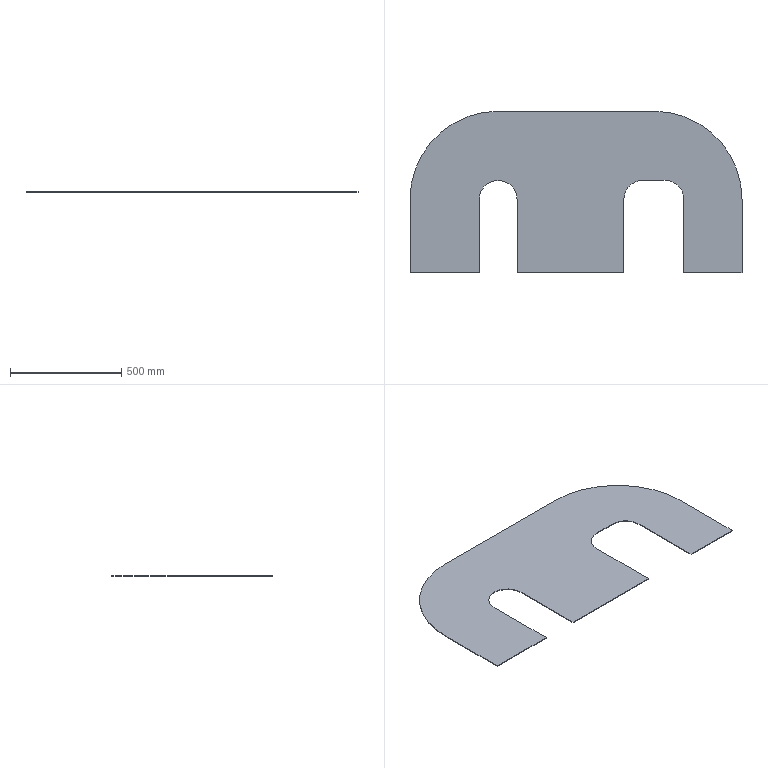Part | NX | features BREP 1 | 1 solid | 18 faces | box 1492 x 726 x 3 mm | volume 2518464 mm3 | plane 13 | cylinder 5 | commonest cylinder face diameters 170 x3 792 x2
STEP:
#1=CARTESIAN_POINT('',(-350.,396.,-1.5));
#2=VERTEX_POINT('',#1);
#3=CARTESIAN_POINT('',(-746.,0.,-1.5));
#4=VERTEX_POINT('',#3);
#5=CARTESIAN_POINT('',(-350.,0.,-1.5));
#6=DIRECTION('',(0.,0.,1.));
#7=DIRECTION('',(1.,0.,0.));
#8=AXIS2_PLACEMENT_3D('',#5,#6,#7);
#9=CIRCLE('',#8,396.);
#10=EDGE_CURVE('',#2,#4,#9,.T.);
#11=ORIENTED_EDGE('',*,*,#10,.T.);
#12=CARTESIAN_POINT('',(-746.,0.,1.5));
#13=VERTEX_POINT('',#12);
#14=CARTESIAN_POINT('',(-746.,0.,1.5));
#15=DIRECTION('',(0.,0.,-1.));
#16=VECTOR('',#15,1000.);
#17=LINE('',#14,#16);
#18=EDGE_CURVE('',#13,#4,#17,.T.);
#19=ORIENTED_EDGE('',*,*,#18,.F.);
#20=CARTESIAN_POINT('',(-350.,396.,1.5));
#21=VERTEX_POINT('',#20);
#22=CARTESIAN_POINT('',(-350.,0.,1.5));
#23=DIRECTION('',(0.,0.,1.));
#24=DIRECTION('',(1.,0.,0.));
#25=AXIS2_PLACEMENT_3D('',#22,#23,#24);
#26=CIRCLE('',#25,396.);
#27=EDGE_CURVE('',#21,#13,#26,.T.);
#28=ORIENTED_EDGE('',*,*,#27,.F.);
#29=CARTESIAN_POINT('',(-350.,396.,1.5));
#30=DIRECTION('',(0.,0.,-1.));
#31=VECTOR('',#30,1000.);
#32=LINE('',#29,#31);
#33=EDGE_CURVE('',#21,#2,#32,.T.);
#34=ORIENTED_EDGE('',*,*,#33,.T.);
#35=EDGE_LOOP('',(#11,#19,#28,#34));
#36=FACE_BOUND('',#35,.T.);
#37=CARTESIAN_POINT('',(-350.,0.,1.5));
#38=DIRECTION('',(0.,0.,-1.));
#39=DIRECTION('',(1.,0.,0.));
#40=AXIS2_PLACEMENT_3D('',#37,#38,#39);
#41=CYLINDRICAL_SURFACE('',#40,396.);
#42=ADVANCED_FACE('',(#36),#41,.T.);
#43=CARTESIAN_POINT('',(-746.,-330.,-1.5));
#44=VERTEX_POINT('',#43);
#45=CARTESIAN_POINT('',(-746.,0.,-1.5));
#46=DIRECTION('',(0.,-1.,0.));
#47=VECTOR('',#46,1000.);
#48=LINE('',#45,#47);
#49=EDGE_CURVE('',#4,#44,#48,.T.);
#50=ORIENTED_EDGE('',*,*,#49,.T.);
#51=CARTESIAN_POINT('',(-746.,-330.,1.5));
#52=VERTEX_POINT('',#51);
#53=CARTESIAN_POINT('',(-746.,-330.,1.5));
#54=DIRECTION('',(0.,0.,-1.));
#55=VECTOR('',#54,1000.);
#56=LINE('',#53,#55);
#57=EDGE_CURVE('',#52,#44,#56,.T.);
#58=ORIENTED_EDGE('',*,*,#57,.F.);
#59=CARTESIAN_POINT('',(-746.,0.,1.5));
#60=DIRECTION('',(0.,-1.,0.));
#61=VECTOR('',#60,1000.);
#62=LINE('',#59,#61);
#63=EDGE_CURVE('',#13,#52,#62,.T.);
#64=ORIENTED_EDGE('',*,*,#63,.F.);
#65=ORIENTED_EDGE('',*,*,#18,.T.);
#66=EDGE_LOOP('',(#50,#58,#64,#65));
#67=FACE_BOUND('',#66,.T.);
#68=CARTESIAN_POINT('',(-746.,0.,1.5));
#69=DIRECTION('',(1.,0.,0.));
#70=DIRECTION('',(0.,0.,1.));
#71=AXIS2_PLACEMENT_3D('',#68,#69,#70);
#72=PLANE('',#71);
#73=ADVANCED_FACE('',(#67),#72,.F.);
#74=CARTESIAN_POINT('',(-435.,-330.,-1.5));
#75=VERTEX_POINT('',#74);
#76=CARTESIAN_POINT('',(-746.,-330.,-1.5));
#77=DIRECTION('',(1.,0.,0.));
#78=VECTOR('',#77,1000.);
#79=LINE('',#76,#78);
#80=EDGE_CURVE('',#44,#75,#79,.T.);
#81=ORIENTED_EDGE('',*,*,#80,.T.);
#82=CARTESIAN_POINT('',(-435.,-330.,1.5));
#83=VERTEX_POINT('',#82);
#84=CARTESIAN_POINT('',(-435.,-330.,1.5));
#85=DIRECTION('',(0.,0.,-1.));
#86=VECTOR('',#85,1000.);
#87=LINE('',#84,#86);
#88=EDGE_CURVE('',#83,#75,#87,.T.);
#89=ORIENTED_EDGE('',*,*,#88,.F.);
#90=CARTESIAN_POINT('',(-746.,-330.,1.5));
#91=DIRECTION('',(1.,0.,0.));
#92=VECTOR('',#91,1000.);
#93=LINE('',#90,#92);
#94=EDGE_CURVE('',#52,#83,#93,.T.);
#95=ORIENTED_EDGE('',*,*,#94,.F.);
#96=ORIENTED_EDGE('',*,*,#57,.T.);
#97=EDGE_LOOP('',(#81,#89,#95,#96));
#98=FACE_BOUND('',#97,.T.);
#99=CARTESIAN_POINT('',(-746.,-330.,1.5));
#100=DIRECTION('',(0.,1.,0.));
#101=DIRECTION('',(1.,0.,0.));
#102=AXIS2_PLACEMENT_3D('',#99,#100,#101);
#103=PLANE('',#102);
#104=ADVANCED_FACE('',(#98),#103,.F.);
#105=CARTESIAN_POINT('',(-435.,0.,-1.5));
#106=VERTEX_POINT('',#105);
#107=CARTESIAN_POINT('',(-435.,0.,-1.5));
#108=DIRECTION('',(0.,1.,0.));
#109=VECTOR('',#108,1000.);
#110=LINE('',#107,#109);
#111=EDGE_CURVE('',#75,#106,#110,.T.);
#112=ORIENTED_EDGE('',*,*,#111,.T.);
#113=CARTESIAN_POINT('',(-435.,0.,1.5));
#114=VERTEX_POINT('',#113);
#115=CARTESIAN_POINT('',(-435.,0.,1.5));
#116=DIRECTION('',(0.,0.,-1.));
#117=VECTOR('',#116,1000.);
#118=LINE('',#115,#117);
#119=EDGE_CURVE('',#114,#106,#118,.T.);
#120=ORIENTED_EDGE('',*,*,#119,.F.);
#121=CARTESIAN_POINT('',(-435.,0.,1.5));
#122=DIRECTION('',(0.,1.,0.));
#123=VECTOR('',#122,1000.);
#124=LINE('',#121,#123);
#125=EDGE_CURVE('',#83,#114,#124,.T.);
#126=ORIENTED_EDGE('',*,*,#125,.F.);
#127=ORIENTED_EDGE('',*,*,#88,.T.);
#128=EDGE_LOOP('',(#112,#120,#126,#127));
#129=FACE_BOUND('',#128,.T.);
#130=CARTESIAN_POINT('',(-435.,0.,1.5));
#131=DIRECTION('',(-1.,0.,0.));
#132=DIRECTION('',(0.,1.,0.));
#133=AXIS2_PLACEMENT_3D('',#130,#131,#132);
#134=PLANE('',#133);
#135=ADVANCED_FACE('',(#129),#134,.F.);
#136=CARTESIAN_POINT('',(-265.,0.,-1.5));
#137=VERTEX_POINT('',#136);
#138=CARTESIAN_POINT('',(-350.,0.,-1.5));
#139=DIRECTION('',(0.,0.,-1.));
#140=DIRECTION('',(1.,0.,0.));
#141=AXIS2_PLACEMENT_3D('',#138,#139,#140);
#142=CIRCLE('',#141,85.);
#143=EDGE_CURVE('',#106,#137,#142,.T.);
#144=ORIENTED_EDGE('',*,*,#143,.T.);
#145=CARTESIAN_POINT('',(-265.,0.,1.5));
#146=VERTEX_POINT('',#145);
#147=CARTESIAN_POINT('',(-265.,0.,1.5));
#148=DIRECTION('',(0.,0.,-1.));
#149=VECTOR('',#148,1000.);
#150=LINE('',#147,#149);
#151=EDGE_CURVE('',#146,#137,#150,.T.);
#152=ORIENTED_EDGE('',*,*,#151,.F.);
#153=CARTESIAN_POINT('',(-350.,0.,1.5));
#154=DIRECTION('',(0.,0.,-1.));
#155=DIRECTION('',(1.,0.,0.));
#156=AXIS2_PLACEMENT_3D('',#153,#154,#155);
#157=CIRCLE('',#156,85.);
#158=EDGE_CURVE('',#114,#146,#157,.T.);
#159=ORIENTED_EDGE('',*,*,#158,.F.);
#160=ORIENTED_EDGE('',*,*,#119,.T.);
#161=EDGE_LOOP('',(#144,#152,#159,#160));
#162=FACE_BOUND('',#161,.T.);
#163=CARTESIAN_POINT('',(-350.,0.,1.5));
#164=DIRECTION('',(0.,0.,-1.));
#165=DIRECTION('',(1.,0.,0.));
#166=AXIS2_PLACEMENT_3D('',#163,#164,#165);
#167=CYLINDRICAL_SURFACE('',#166,85.);
#168=ADVANCED_FACE('',(#162),#167,.F.);
#169=CARTESIAN_POINT('',(-265.,-330.,-1.5));
#170=VERTEX_POINT('',#169);
#171=CARTESIAN_POINT('',(-265.,0.,-1.5));
#172=DIRECTION('',(0.,-1.,0.));
#173=VECTOR('',#172,1000.);
#174=LINE('',#171,#173);
#175=EDGE_CURVE('',#137,#170,#174,.T.);
#176=ORIENTED_EDGE('',*,*,#175,.T.);
#177=CARTESIAN_POINT('',(-265.,-330.,1.5));
#178=VERTEX_POINT('',#177);
#179=CARTESIAN_POINT('',(-265.,-330.,1.5));
#180=DIRECTION('',(0.,0.,-1.));
#181=VECTOR('',#180,1000.);
#182=LINE('',#179,#181);
#183=EDGE_CURVE('',#178,#170,#182,.T.);
#184=ORIENTED_EDGE('',*,*,#183,.F.);
#185=CARTESIAN_POINT('',(-265.,0.,1.5));
#186=DIRECTION('',(0.,-1.,0.));
#187=VECTOR('',#186,1000.);
#188=LINE('',#185,#187);
#189=EDGE_CURVE('',#146,#178,#188,.T.);
#190=ORIENTED_EDGE('',*,*,#189,.F.);
#191=ORIENTED_EDGE('',*,*,#151,.T.);
#192=EDGE_LOOP('',(#176,#184,#190,#191));
#193=FACE_BOUND('',#192,.T.);
#194=CARTESIAN_POINT('',(-265.,0.,1.5));
#195=DIRECTION('',(1.,0.,0.));
#196=DIRECTION('',(0.,-1.,0.));
#197=AXIS2_PLACEMENT_3D('',#194,#195,#196);
#198=PLANE('',#197);
#199=ADVANCED_FACE('',(#193),#198,.F.);
#200=CARTESIAN_POINT('',(215.,-330.,-1.5));
#201=VERTEX_POINT('',#200);
#202=CARTESIAN_POINT('',(-265.,-330.,-1.5));
#203=DIRECTION('',(1.,0.,0.));
#204=VECTOR('',#203,1000.);
#205=LINE('',#202,#204);
#206=EDGE_CURVE('',#170,#201,#205,.T.);
#207=ORIENTED_EDGE('',*,*,#206,.T.);
#208=CARTESIAN_POINT('',(215.,-330.,1.5));
#209=VERTEX_POINT('',#208);
#210=CARTESIAN_POINT('',(215.,-330.,1.5));
#211=DIRECTION('',(0.,0.,-1.));
#212=VECTOR('',#211,1000.);
#213=LINE('',#210,#212);
#214=EDGE_CURVE('',#209,#201,#213,.T.);
#215=ORIENTED_EDGE('',*,*,#214,.F.);
#216=CARTESIAN_POINT('',(-265.,-330.,1.5));
#217=DIRECTION('',(1.,0.,0.));
#218=VECTOR('',#217,1000.);
#219=LINE('',#216,#218);
#220=EDGE_CURVE('',#178,#209,#219,.T.);
#221=ORIENTED_EDGE('',*,*,#220,.F.);
#222=ORIENTED_EDGE('',*,*,#183,.T.);
#223=EDGE_LOOP('',(#207,#215,#221,#222));
#224=FACE_BOUND('',#223,.T.);
#225=CARTESIAN_POINT('',(-265.,-330.,1.5));
#226=DIRECTION('',(0.,1.,0.));
#227=DIRECTION('',(0.,0.,-1.));
#228=AXIS2_PLACEMENT_3D('',#225,#226,#227);
#229=PLANE('',#228);
#230=ADVANCED_FACE('',(#224),#229,.F.);
#231=CARTESIAN_POINT('',(215.,0.,-1.5));
#232=VERTEX_POINT('',#231);
#233=CARTESIAN_POINT('',(215.,0.,-1.5));
#234=DIRECTION('',(0.,1.,0.));
#235=VECTOR('',#234,1000.);
#236=LINE('',#233,#235);
#237=EDGE_CURVE('',#201,#232,#236,.T.);
#238=ORIENTED_EDGE('',*,*,#237,.T.);
#239=CARTESIAN_POINT('',(215.,0.,1.5));
#240=VERTEX_POINT('',#239);
#241=CARTESIAN_POINT('',(215.,0.,1.5));
#242=DIRECTION('',(0.,0.,-1.));
#243=VECTOR('',#242,1000.);
#244=LINE('',#241,#243);
#245=EDGE_CURVE('',#240,#232,#244,.T.);
#246=ORIENTED_EDGE('',*,*,#245,.F.);
#247=CARTESIAN_POINT('',(215.,0.,1.5));
#248=DIRECTION('',(0.,1.,0.));
#249=VECTOR('',#248,1000.);
#250=LINE('',#247,#249);
#251=EDGE_CURVE('',#209,#240,#250,.T.);
#252=ORIENTED_EDGE('',*,*,#251,.F.);
#253=ORIENTED_EDGE('',*,*,#214,.T.);
#254=EDGE_LOOP('',(#238,#246,#252,#253));
#255=FACE_BOUND('',#254,.T.);
#256=CARTESIAN_POINT('',(215.,0.,1.5));
#257=DIRECTION('',(-1.,0.,0.));
#258=DIRECTION('',(0.,1.,0.));
#259=AXIS2_PLACEMENT_3D('',#256,#257,#258);
#260=PLANE('',#259);
#261=ADVANCED_FACE('',(#255),#260,.F.);
#262=CARTESIAN_POINT('',(300.,85.,-1.5));
#263=VERTEX_POINT('',#262);
#264=CARTESIAN_POINT('',(300.,0.,-1.5));
#265=DIRECTION('',(0.,0.,-1.));
#266=DIRECTION('',(1.,0.,0.));
#267=AXIS2_PLACEMENT_3D('',#264,#265,#266);
#268=CIRCLE('',#267,85.);
#269=EDGE_CURVE('',#232,#263,#268,.T.);
#270=ORIENTED_EDGE('',*,*,#269,.T.);
#271=CARTESIAN_POINT('',(300.,85.,1.5));
#272=VERTEX_POINT('',#271);
#273=CARTESIAN_POINT('',(300.,85.,1.5));
#274=DIRECTION('',(0.,0.,-1.));
#275=VECTOR('',#274,1000.);
#276=LINE('',#273,#275);
#277=EDGE_CURVE('',#272,#263,#276,.T.);
#278=ORIENTED_EDGE('',*,*,#277,.F.);
#279=CARTESIAN_POINT('',(300.,0.,1.5));
#280=DIRECTION('',(0.,0.,-1.));
#281=DIRECTION('',(1.,0.,0.));
#282=AXIS2_PLACEMENT_3D('',#279,#280,#281);
#283=CIRCLE('',#282,85.);
#284=EDGE_CURVE('',#240,#272,#283,.T.);
#285=ORIENTED_EDGE('',*,*,#284,.F.);
#286=ORIENTED_EDGE('',*,*,#245,.T.);
#287=EDGE_LOOP('',(#270,#278,#285,#286));
#288=FACE_BOUND('',#287,.T.);
#289=CARTESIAN_POINT('',(300.,0.,1.5));
#290=DIRECTION('',(0.,0.,-1.));
#291=DIRECTION('',(1.,0.,0.));
#292=AXIS2_PLACEMENT_3D('',#289,#290,#291);
#293=CYLINDRICAL_SURFACE('',#292,85.);
#294=ADVANCED_FACE('',(#288),#293,.F.);
#295=CARTESIAN_POINT('',(400.,85.,-1.5));
#296=VERTEX_POINT('',#295);
#297=CARTESIAN_POINT('',(300.,85.,-1.5));
#298=DIRECTION('',(1.,0.,0.));
#299=VECTOR('',#298,1000.);
#300=LINE('',#297,#299);
#301=EDGE_CURVE('',#263,#296,#300,.T.);
#302=ORIENTED_EDGE('',*,*,#301,.T.);
#303=CARTESIAN_POINT('',(400.,85.,1.5));
#304=VERTEX_POINT('',#303);
#305=CARTESIAN_POINT('',(400.,85.,1.5));
#306=DIRECTION('',(0.,0.,-1.));
#307=VECTOR('',#306,1000.);
#308=LINE('',#305,#307);
#309=EDGE_CURVE('',#304,#296,#308,.T.);
#310=ORIENTED_EDGE('',*,*,#309,.F.);
#311=CARTESIAN_POINT('',(300.,85.,1.5));
#312=DIRECTION('',(1.,0.,0.));
#313=VECTOR('',#312,1000.);
#314=LINE('',#311,#313);
#315=EDGE_CURVE('',#272,#304,#314,.T.);
#316=ORIENTED_EDGE('',*,*,#315,.F.);
#317=ORIENTED_EDGE('',*,*,#277,.T.);
#318=EDGE_LOOP('',(#302,#310,#316,#317));
#319=FACE_BOUND('',#318,.T.);
#320=CARTESIAN_POINT('',(300.,85.,1.5));
#321=DIRECTION('',(0.,1.,0.));
#322=DIRECTION('',(0.,0.,-1.));
#323=AXIS2_PLACEMENT_3D('',#320,#321,#322);
#324=PLANE('',#323);
#325=ADVANCED_FACE('',(#319),#324,.F.);
#326=CARTESIAN_POINT('',(485.,0.,-1.5));
#327=VERTEX_POINT('',#326);
#328=CARTESIAN_POINT('',(400.,0.,-1.5));
#329=DIRECTION('',(0.,0.,-1.));
#330=DIRECTION('',(-1.,0.,0.));
#331=AXIS2_PLACEMENT_3D('',#328,#329,#330);
#332=CIRCLE('',#331,85.);
#333=EDGE_CURVE('',#296,#327,#332,.T.);
#334=ORIENTED_EDGE('',*,*,#333,.T.);
#335=CARTESIAN_POINT('',(485.,0.,1.5));
#336=VERTEX_POINT('',#335);
#337=CARTESIAN_POINT('',(485.,0.,1.5));
#338=DIRECTION('',(0.,0.,-1.));
#339=VECTOR('',#338,1000.);
#340=LINE('',#337,#339);
#341=EDGE_CURVE('',#336,#327,#340,.T.);
#342=ORIENTED_EDGE('',*,*,#341,.F.);
#343=CARTESIAN_POINT('',(400.,0.,1.5));
#344=DIRECTION('',(0.,0.,-1.));
#345=DIRECTION('',(-1.,0.,0.));
#346=AXIS2_PLACEMENT_3D('',#343,#344,#345);
#347=CIRCLE('',#346,85.);
#348=EDGE_CURVE('',#304,#336,#347,.T.);
#349=ORIENTED_EDGE('',*,*,#348,.F.);
#350=ORIENTED_EDGE('',*,*,#309,.T.);
#351=EDGE_LOOP('',(#334,#342,#349,#350));
#352=FACE_BOUND('',#351,.T.);
#353=CARTESIAN_POINT('',(400.,0.,1.5));
#354=DIRECTION('',(0.,0.,-1.));
#355=DIRECTION('',(1.,0.,0.));
#356=AXIS2_PLACEMENT_3D('',#353,#354,#355);
#357=CYLINDRICAL_SURFACE('',#356,85.);
#358=ADVANCED_FACE('',(#352),#357,.F.);
#359=CARTESIAN_POINT('',(485.,-330.,-1.5));
#360=VERTEX_POINT('',#359);
#361=CARTESIAN_POINT('',(485.,0.,-1.5));
#362=DIRECTION('',(0.,-1.,0.));
#363=VECTOR('',#362,1000.);
#364=LINE('',#361,#363);
#365=EDGE_CURVE('',#327,#360,#364,.T.);
#366=ORIENTED_EDGE('',*,*,#365,.T.);
#367=CARTESIAN_POINT('',(485.,-330.,1.5));
#368=VERTEX_POINT('',#367);
#369=CARTESIAN_POINT('',(485.,-330.,1.5));
#370=DIRECTION('',(0.,0.,-1.));
#371=VECTOR('',#370,1000.);
#372=LINE('',#369,#371);
#373=EDGE_CURVE('',#368,#360,#372,.T.);
#374=ORIENTED_EDGE('',*,*,#373,.F.);
#375=CARTESIAN_POINT('',(485.,0.,1.5));
#376=DIRECTION('',(0.,-1.,0.));
#377=VECTOR('',#376,1000.);
#378=LINE('',#375,#377);
#379=EDGE_CURVE('',#336,#368,#378,.T.);
#380=ORIENTED_EDGE('',*,*,#379,.F.);
#381=ORIENTED_EDGE('',*,*,#341,.T.);
#382=EDGE_LOOP('',(#366,#374,#380,#381));
#383=FACE_BOUND('',#382,.T.);
#384=CARTESIAN_POINT('',(485.,0.,1.5));
#385=DIRECTION('',(1.,0.,0.));
#386=DIRECTION('',(0.,0.,1.));
#387=AXIS2_PLACEMENT_3D('',#384,#385,#386);
#388=PLANE('',#387);
#389=ADVANCED_FACE('',(#383),#388,.F.);
#390=CARTESIAN_POINT('',(746.,-330.,-1.5));
#391=VERTEX_POINT('',#390);
#392=CARTESIAN_POINT('',(485.,-330.,-1.5));
#393=DIRECTION('',(1.,0.,0.));
#394=VECTOR('',#393,1000.);
#395=LINE('',#392,#394);
#396=EDGE_CURVE('',#360,#391,#395,.T.);
#397=ORIENTED_EDGE('',*,*,#396,.T.);
#398=CARTESIAN_POINT('',(746.,-330.,1.5));
#399=VERTEX_POINT('',#398);
#400=CARTESIAN_POINT('',(746.,-330.,1.5));
#401=DIRECTION('',(0.,0.,-1.));
#402=VECTOR('',#401,1000.);
#403=LINE('',#400,#402);
#404=EDGE_CURVE('',#399,#391,#403,.T.);
#405=ORIENTED_EDGE('',*,*,#404,.F.);
#406=CARTESIAN_POINT('',(485.,-330.,1.5));
#407=DIRECTION('',(1.,0.,0.));
#408=VECTOR('',#407,1000.);
#409=LINE('',#406,#408);
#410=EDGE_CURVE('',#368,#399,#409,.T.);
#411=ORIENTED_EDGE('',*,*,#410,.F.);
#412=ORIENTED_EDGE('',*,*,#373,.T.);
#413=EDGE_LOOP('',(#397,#405,#411,#412));
#414=FACE_BOUND('',#413,.T.);
#415=CARTESIAN_POINT('',(485.,-330.,1.5));
#416=DIRECTION('',(0.,1.,0.));
#417=DIRECTION('',(0.,0.,-1.));
#418=AXIS2_PLACEMENT_3D('',#415,#416,#417);
#419=PLANE('',#418);
#420=ADVANCED_FACE('',(#414),#419,.F.);
#421=CARTESIAN_POINT('',(746.,0.,-1.5));
#422=VERTEX_POINT('',#421);
#423=CARTESIAN_POINT('',(746.,0.,-1.5));
#424=DIRECTION('',(0.,1.,0.));
#425=VECTOR('',#424,1000.);
#426=LINE('',#423,#425);
#427=EDGE_CURVE('',#391,#422,#426,.T.);
#428=ORIENTED_EDGE('',*,*,#427,.T.);
#429=CARTESIAN_POINT('',(746.,0.,1.5));
#430=VERTEX_POINT('',#429);
#431=CARTESIAN_POINT('',(746.,0.,1.5));
#432=DIRECTION('',(0.,0.,-1.));
#433=VECTOR('',#432,1000.);
#434=LINE('',#431,#433);
#435=EDGE_CURVE('',#430,#422,#434,.T.);
#436=ORIENTED_EDGE('',*,*,#435,.F.);
#437=CARTESIAN_POINT('',(746.,0.,1.5));
#438=DIRECTION('',(0.,1.,0.));
#439=VECTOR('',#438,1000.);
#440=LINE('',#437,#439);
#441=EDGE_CURVE('',#399,#430,#440,.T.);
#442=ORIENTED_EDGE('',*,*,#441,.F.);
#443=ORIENTED_EDGE('',*,*,#404,.T.);
#444=EDGE_LOOP('',(#428,#436,#442,#443));
#445=FACE_BOUND('',#444,.T.);
#446=CARTESIAN_POINT('',(746.,0.,1.5));
#447=DIRECTION('',(-1.,0.,0.));
#448=DIRECTION('',(0.,0.,-1.));
#449=AXIS2_PLACEMENT_3D('',#446,#447,#448);
#450=PLANE('',#449);
#451=ADVANCED_FACE('',(#445),#450,.F.);
#452=CARTESIAN_POINT('',(350.,396.,-1.5));
#453=VERTEX_POINT('',#452);
#454=CARTESIAN_POINT('',(350.,0.,-1.5));
#455=DIRECTION('',(0.,0.,1.));
#456=DIRECTION('',(-1.,0.,0.));
#457=AXIS2_PLACEMENT_3D('',#454,#455,#456);
#458=CIRCLE('',#457,396.);
#459=EDGE_CURVE('',#422,#453,#458,.T.);
#460=ORIENTED_EDGE('',*,*,#459,.T.);
#461=CARTESIAN_POINT('',(350.,396.,1.5));
#462=VERTEX_POINT('',#461);
#463=CARTESIAN_POINT('',(350.,396.,1.5));
#464=DIRECTION('',(0.,0.,-1.));
#465=VECTOR('',#464,1000.);
#466=LINE('',#463,#465);
#467=EDGE_CURVE('',#462,#453,#466,.T.);
#468=ORIENTED_EDGE('',*,*,#467,.F.);
#469=CARTESIAN_POINT('',(350.,0.,1.5));
#470=DIRECTION('',(0.,0.,1.));
#471=DIRECTION('',(-1.,0.,0.));
#472=AXIS2_PLACEMENT_3D('',#469,#470,#471);
#473=CIRCLE('',#472,396.);
#474=EDGE_CURVE('',#430,#462,#473,.T.);
#475=ORIENTED_EDGE('',*,*,#474,.F.);
#476=ORIENTED_EDGE('',*,*,#435,.T.);
#477=EDGE_LOOP('',(#460,#468,#475,#476));
#478=FACE_BOUND('',#477,.T.);
#479=CARTESIAN_POINT('',(350.,0.,1.5));
#480=DIRECTION('',(0.,0.,-1.));
#481=DIRECTION('',(1.,0.,0.));
#482=AXIS2_PLACEMENT_3D('',#479,#480,#481);
#483=CYLINDRICAL_SURFACE('',#482,396.);
#484=ADVANCED_FACE('',(#478),#483,.T.);
#485=CARTESIAN_POINT('',(-350.,396.,-1.5));
#486=DIRECTION('',(-1.,0.,0.));
#487=VECTOR('',#486,1000.);
#488=LINE('',#485,#487);
#489=EDGE_CURVE('',#453,#2,#488,.T.);
#490=ORIENTED_EDGE('',*,*,#489,.T.);
#491=ORIENTED_EDGE('',*,*,#33,.F.);
#492=CARTESIAN_POINT('',(-350.,396.,1.5));
#493=DIRECTION('',(-1.,0.,0.));
#494=VECTOR('',#493,1000.);
#495=LINE('',#492,#494);
#496=EDGE_CURVE('',#462,#21,#495,.T.);
#497=ORIENTED_EDGE('',*,*,#496,.F.);
#498=ORIENTED_EDGE('',*,*,#467,.T.);
#499=EDGE_LOOP('',(#490,#491,#497,#498));
#500=FACE_BOUND('',#499,.T.);
#501=CARTESIAN_POINT('',(-350.,396.,1.5));
#502=DIRECTION('',(0.,-1.,0.));
#503=DIRECTION('',(-1.,0.,0.));
#504=AXIS2_PLACEMENT_3D('',#501,#502,#503);
#505=PLANE('',#504);
#506=ADVANCED_FACE('',(#500),#505,.F.);
#507=ORIENTED_EDGE('',*,*,#27,.T.);
#508=ORIENTED_EDGE('',*,*,#63,.T.);
#509=ORIENTED_EDGE('',*,*,#94,.T.);
#510=ORIENTED_EDGE('',*,*,#125,.T.);
#511=ORIENTED_EDGE('',*,*,#158,.T.);
#512=ORIENTED_EDGE('',*,*,#189,.T.);
#513=ORIENTED_EDGE('',*,*,#220,.T.);
#514=ORIENTED_EDGE('',*,*,#251,.T.);
#515=ORIENTED_EDGE('',*,*,#284,.T.);
#516=ORIENTED_EDGE('',*,*,#315,.T.);
#517=ORIENTED_EDGE('',*,*,#348,.T.);
#518=ORIENTED_EDGE('',*,*,#379,.T.);
#519=ORIENTED_EDGE('',*,*,#410,.T.);
#520=ORIENTED_EDGE('',*,*,#441,.T.);
#521=ORIENTED_EDGE('',*,*,#474,.T.);
#522=ORIENTED_EDGE('',*,*,#496,.T.);
#523=EDGE_LOOP('',(#507,#508,#509,#510,#511,#512,#513,#514,#515,#516,#517,#518,#519,#520,#521,#522));
#524=FACE_BOUND('',#523,.T.);
#525=CARTESIAN_POINT('',(-350.,0.,1.5));
#526=DIRECTION('',(0.,0.,1.));
#527=DIRECTION('',(-1.,0.,0.));
#528=AXIS2_PLACEMENT_3D('',#525,#526,#527);
#529=PLANE('',#528);
#530=ADVANCED_FACE('',(#524),#529,.T.);
#531=ORIENTED_EDGE('',*,*,#10,.F.);
#532=ORIENTED_EDGE('',*,*,#489,.F.);
#533=ORIENTED_EDGE('',*,*,#459,.F.);
#534=ORIENTED_EDGE('',*,*,#427,.F.);
#535=ORIENTED_EDGE('',*,*,#396,.F.);
#536=ORIENTED_EDGE('',*,*,#365,.F.);
#537=ORIENTED_EDGE('',*,*,#333,.F.);
#538=ORIENTED_EDGE('',*,*,#301,.F.);
#539=ORIENTED_EDGE('',*,*,#269,.F.);
#540=ORIENTED_EDGE('',*,*,#237,.F.);
#541=ORIENTED_EDGE('',*,*,#206,.F.);
#542=ORIENTED_EDGE('',*,*,#175,.F.);
#543=ORIENTED_EDGE('',*,*,#143,.F.);
#544=ORIENTED_EDGE('',*,*,#111,.F.);
#545=ORIENTED_EDGE('',*,*,#80,.F.);
#546=ORIENTED_EDGE('',*,*,#49,.F.);
#547=EDGE_LOOP('',(#531,#532,#533,#534,#535,#536,#537,#538,#539,#540,#541,#542,#543,#544,#545,#546));
#548=FACE_BOUND('',#547,.T.);
#549=CARTESIAN_POINT('',(-350.,0.,-1.5));
#550=DIRECTION('',(0.,0.,1.));
#551=DIRECTION('',(-1.,0.,0.));
#552=AXIS2_PLACEMENT_3D('',#549,#550,#551);
#553=PLANE('',#552);
#554=ADVANCED_FACE('',(#548),#553,.F.);
#555=CLOSED_SHELL('',(#42,#73,#104,#135,#168,#199,#230,#261,#294,#325,#358,#389,#420,#451,#484,#506,#530,#554));
#556=MANIFOLD_SOLID_BREP('',#555);
#557=(LENGTH_UNIT()NAMED_UNIT(*)SI_UNIT(.MILLI.,.METRE.));
#558=UNCERTAINTY_MEASURE_WITH_UNIT(LENGTH_MEASURE(0.00001),#557,'','');
#559=(NAMED_UNIT(*)PLANE_ANGLE_UNIT()SI_UNIT($,.RADIAN.));
#560=(NAMED_UNIT(*)SI_UNIT($,.STERADIAN.)SOLID_ANGLE_UNIT());
#561=(GEOMETRIC_REPRESENTATION_CONTEXT(3)GLOBAL_UNCERTAINTY_ASSIGNED_CONTEXT((#558))GLOBAL_UNIT_ASSIGNED_CONTEXT((#557,#559,#560))REPRESENTATION_CONTEXT('',''));
#562=ADVANCED_BREP_SHAPE_REPRESENTATION('',(#556),#561);